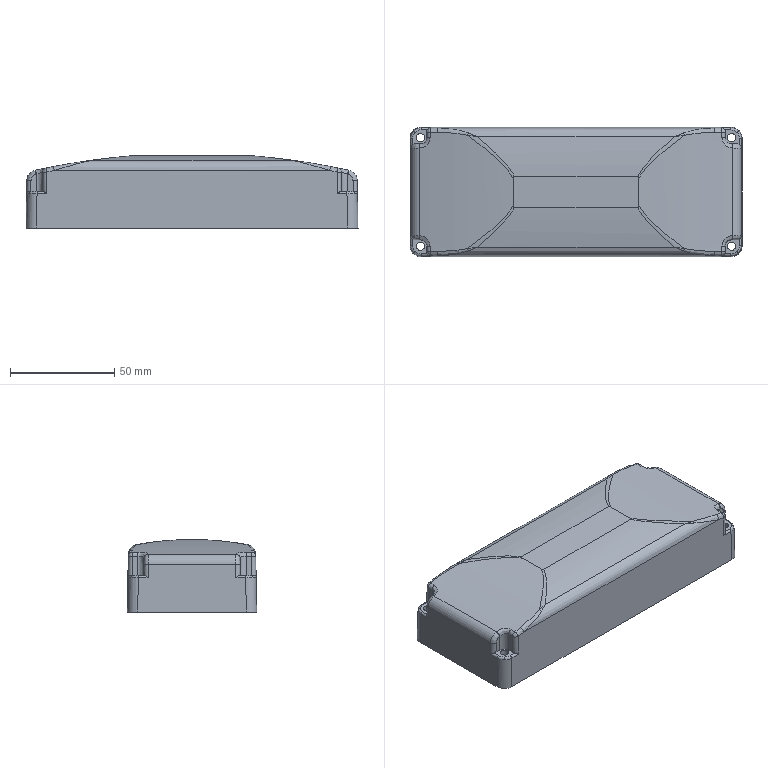Part | SolidWorks | features BaseBody 1 | 1 solid | 141 faces | box 159 x 62 x 34.528 mm | volume 50117 mm3 | cylinder 62 | spline 44 | plane 35 | commonest cylinder face diameters 4 x20 2 x8 10 x8 8.6 x6 5.4 x4 6 x4